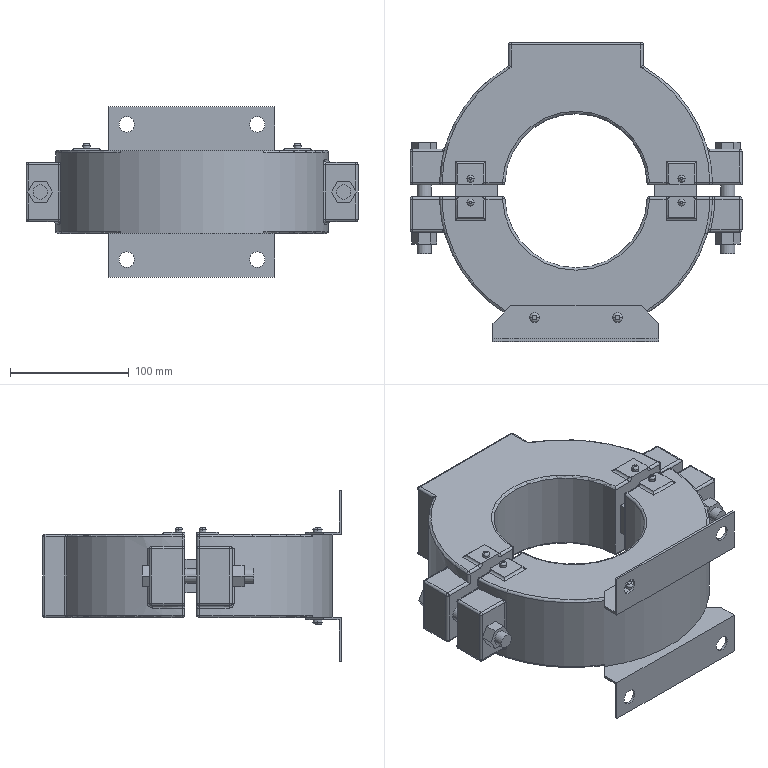Part | STEP file | LXZK120 | 1 solid | 314 faces | box 280 x 252 x 144 mm | volume 2421478 mm3 | cylinder 121 | plane 97 | torus 40 | sphere 34 | spline 14 | other 8 | commonest cylinder face diameters 4 x84 6 x8 8 x8 12 x8 13 x8 230 x3